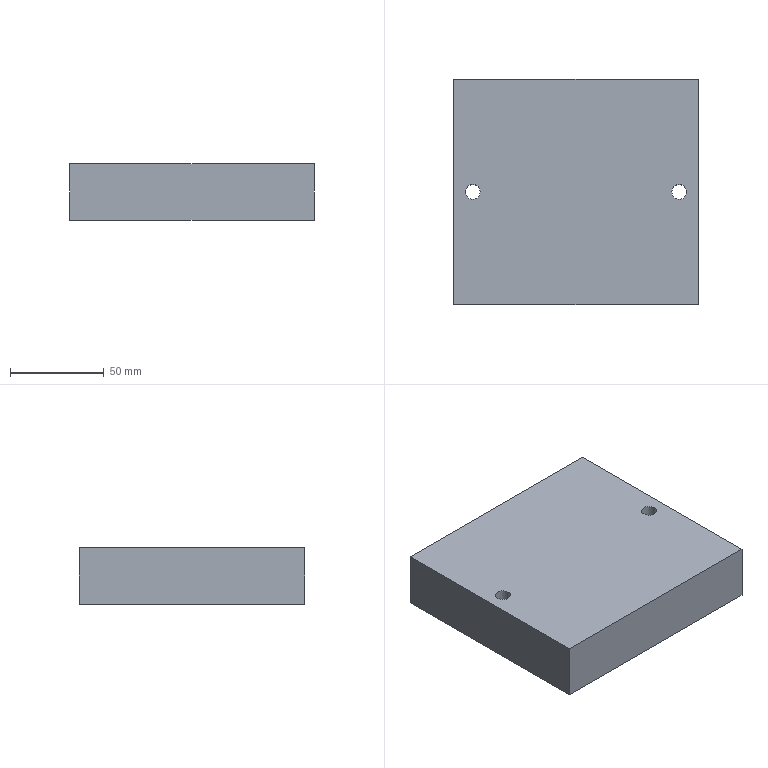Part | STEP file | YBQDJ-YL-7 | 1 solid | 8 faces | box 130 x 120 x 30 mm | volume 464984 mm3 | plane 6 | cylinder 2 | commonest cylinder face diameters 8 x2
STEP:
#1=CARTESIAN_POINT('',(0.,0.,0.));
#2=DIRECTION('',(0.,0.,1.));
#3=DIRECTION('',(1.,0.,0.));
#4=AXIS2_PLACEMENT_3D('',#1,#2,#3);
#5=CARTESIAN_POINT('',(255.5,-195.,95.));
#6=VERTEX_POINT('',#5);
#7=CARTESIAN_POINT('',(247.5,-195.,95.));
#8=VERTEX_POINT('',#7);
#9=CARTESIAN_POINT('',(251.5,-195.,95.));
#10=DIRECTION('',(0.,0.,-1.));
#11=DIRECTION('',(1.,0.,0.));
#12=AXIS2_PLACEMENT_3D('',#9,#10,#11);
#13=CIRCLE('',#12,4.);
#14=CARTESIAN_POINT('',(251.5,-195.,28.));
#15=DIRECTION('',(0.,0.,1.));
#16=DIRECTION('',(-1.,0.,0.));
#17=AXIS2_PLACEMENT_3D('',#14,#15,#16);
#18=CYLINDRICAL_SURFACE('',#17,4.);
#19=CARTESIAN_POINT('',(3.142,67.));
#20=DIRECTION('',(-1.,0.));
#21=VECTOR('',#20,1.);
#22=LINE('',#19,#21);
#23=(GEOMETRIC_REPRESENTATION_CONTEXT(2)PARAMETRIC_REPRESENTATION_CONTEXT()REPRESENTATION_CONTEXT('',''));
#24=DEFINITIONAL_REPRESENTATION('',(#22),#23);
#25=PCURVE('',#18,#24);
#26=CARTESIAN_POINT('',(343.5,-115.,95.));
#27=DIRECTION('',(0.,0.,1.));
#28=DIRECTION('',(1.,0.,0.));
#29=AXIS2_PLACEMENT_3D('',#26,#27,#28);
#30=PLANE('',#29);
#31=CARTESIAN_POINT('',(-88.,-80.));
#32=CARTESIAN_POINT('',(-88.,-86.928));
#33=CARTESIAN_POINT('',(-94.,-83.464));
#34=CARTESIAN_POINT('',(-100.,-80.));
#35=CARTESIAN_POINT('',(-94.,-76.536));
#36=CARTESIAN_POINT('',(-88.,-73.072));
#37=CARTESIAN_POINT('',(-88.,-80.));
#38=(BOUNDED_CURVE()B_SPLINE_CURVE(2,(#31,#32,#33,#34,#35,#36,#37),.UNSPECIFIED.,.T.,.F.)B_SPLINE_CURVE_WITH_KNOTS((1,2,2,2,2,1),(-2.094,0.,2.094,4.189,6.283,8.378),.UNSPECIFIED.)CURVE()GEOMETRIC_REPRESENTATION_ITEM()RATIONAL_B_SPLINE_CURVE((1.,0.5,1.,0.5,1.,0.5,1.))REPRESENTATION_ITEM(''));
#39=(GEOMETRIC_REPRESENTATION_CONTEXT(2)PARAMETRIC_REPRESENTATION_CONTEXT()REPRESENTATION_CONTEXT('',''));
#40=DEFINITIONAL_REPRESENTATION('',(#38),#39);
#41=PCURVE('',#30,#40);
#42=SURFACE_CURVE('',#13,(#25,#41),.PCURVE_S1.);
#43=EDGE_CURVE('',#6,#8,#42,.T.);
#44=ORIENTED_EDGE('',*,*,#43,.T.);
#45=CARTESIAN_POINT('',(247.5,-195.,65.));
#46=VERTEX_POINT('',#45);
#47=CARTESIAN_POINT('',(247.5,-195.,65.));
#48=CARTESIAN_POINT('',(247.5,-195.,95.));
#49=B_SPLINE_CURVE_WITH_KNOTS('',1,(#47,#48),.UNSPECIFIED.,.F.,.F.,(2,2),(37.,67.),.PIECEWISE_BEZIER_KNOTS.);
#50=CARTESIAN_POINT('',(0.,0.));
#51=DIRECTION('',(0.,1.));
#52=VECTOR('',#51,1.);
#53=LINE('',#50,#52);
#54=(GEOMETRIC_REPRESENTATION_CONTEXT(2)PARAMETRIC_REPRESENTATION_CONTEXT()REPRESENTATION_CONTEXT('',''));
#55=DEFINITIONAL_REPRESENTATION('',(#53),#54);
#56=PCURVE('',#18,#55);
#57=CARTESIAN_POINT('',(6.283,0.));
#58=DIRECTION('',(0.,1.));
#59=VECTOR('',#58,1.);
#60=LINE('',#57,#59);
#61=(GEOMETRIC_REPRESENTATION_CONTEXT(2)PARAMETRIC_REPRESENTATION_CONTEXT()REPRESENTATION_CONTEXT('',''));
#62=DEFINITIONAL_REPRESENTATION('',(#60),#61);
#63=PCURVE('',#18,#62);
#64=SEAM_CURVE('',#49,(#56,#63),.PCURVE_S1.);
#65=EDGE_CURVE('',#46,#8,#64,.T.);
#66=ORIENTED_EDGE('',*,*,#65,.F.);
#67=CARTESIAN_POINT('',(251.5,-195.,65.));
#68=DIRECTION('',(0.,0.,1.));
#69=DIRECTION('',(-1.,0.,0.));
#70=AXIS2_PLACEMENT_3D('',#67,#68,#69);
#71=CIRCLE('',#70,4.);
#72=CARTESIAN_POINT('',(0.,37.));
#73=DIRECTION('',(1.,0.));
#74=VECTOR('',#73,1.);
#75=LINE('',#72,#74);
#76=(GEOMETRIC_REPRESENTATION_CONTEXT(2)PARAMETRIC_REPRESENTATION_CONTEXT()REPRESENTATION_CONTEXT('',''));
#77=DEFINITIONAL_REPRESENTATION('',(#75),#76);
#78=PCURVE('',#18,#77);
#79=CARTESIAN_POINT('',(343.5,-115.,65.));
#80=DIRECTION('',(0.,0.,1.));
#81=DIRECTION('',(1.,0.,0.));
#82=AXIS2_PLACEMENT_3D('',#79,#80,#81);
#83=PLANE('',#82);
#84=CARTESIAN_POINT('',(-92.,-80.));
#85=DIRECTION('',(-1.,0.));
#86=AXIS2_PLACEMENT_2D('',#84,#85);
#87=CIRCLE('',#86,4.);
#88=(GEOMETRIC_REPRESENTATION_CONTEXT(2)PARAMETRIC_REPRESENTATION_CONTEXT()REPRESENTATION_CONTEXT('',''));
#89=DEFINITIONAL_REPRESENTATION('',(#87),#88);
#90=PCURVE('',#83,#89);
#91=SURFACE_CURVE('',#71,(#78,#90),.PCURVE_S1.);
#92=EDGE_CURVE('',#46,#46,#91,.T.);
#93=ORIENTED_EDGE('',*,*,#92,.T.);
#94=ORIENTED_EDGE('',*,*,#65,.T.);
#95=CARTESIAN_POINT('',(251.5,-195.,95.));
#96=DIRECTION('',(0.,0.,-1.));
#97=DIRECTION('',(1.,0.,0.));
#98=AXIS2_PLACEMENT_3D('',#95,#96,#97);
#99=CIRCLE('',#98,4.);
#100=CARTESIAN_POINT('',(9.425,67.));
#101=DIRECTION('',(-1.,0.));
#102=VECTOR('',#101,1.);
#103=LINE('',#100,#102);
#104=(GEOMETRIC_REPRESENTATION_CONTEXT(2)PARAMETRIC_REPRESENTATION_CONTEXT()REPRESENTATION_CONTEXT('',''));
#105=DEFINITIONAL_REPRESENTATION('',(#103),#104);
#106=PCURVE('',#18,#105);
#107=CARTESIAN_POINT('',(-88.,-80.));
#108=CARTESIAN_POINT('',(-88.,-86.928));
#109=CARTESIAN_POINT('',(-94.,-83.464));
#110=CARTESIAN_POINT('',(-100.,-80.));
#111=CARTESIAN_POINT('',(-94.,-76.536));
#112=CARTESIAN_POINT('',(-88.,-73.072));
#113=CARTESIAN_POINT('',(-88.,-80.));
#114=(BOUNDED_CURVE()B_SPLINE_CURVE(2,(#107,#108,#109,#110,#111,#112,#113),.UNSPECIFIED.,.T.,.F.)B_SPLINE_CURVE_WITH_KNOTS((1,2,2,2,2,1),(-2.094,0.,2.094,4.189,6.283,8.378),.UNSPECIFIED.)CURVE()GEOMETRIC_REPRESENTATION_ITEM()RATIONAL_B_SPLINE_CURVE((1.,0.5,1.,0.5,1.,0.5,1.))REPRESENTATION_ITEM(''));
#115=(GEOMETRIC_REPRESENTATION_CONTEXT(2)PARAMETRIC_REPRESENTATION_CONTEXT()REPRESENTATION_CONTEXT('',''));
#116=DEFINITIONAL_REPRESENTATION('',(#114),#115);
#117=PCURVE('',#30,#116);
#118=SURFACE_CURVE('',#99,(#106,#117),.PCURVE_S1.);
#119=EDGE_CURVE('',#8,#6,#118,.T.);
#120=ORIENTED_EDGE('',*,*,#119,.T.);
#121=EDGE_LOOP('',(#44,#66,#93,#94,#120));
#122=FACE_BOUND('',#121,.F.);
#123=ADVANCED_FACE('',(#122),#18,.F.);
#124=CARTESIAN_POINT('',(241.5,-135.,95.));
#125=VERTEX_POINT('',#124);
#126=CARTESIAN_POINT('',(241.5,-135.,65.));
#127=VERTEX_POINT('',#126);
#128=CARTESIAN_POINT('',(241.5,-135.,108.));
#129=DIRECTION('',(0.,0.,-1.));
#130=VECTOR('',#129,1.);
#131=LINE('',#128,#130);
#132=CARTESIAN_POINT('',(241.5,-90.,108.));
#133=DIRECTION('',(1.,0.,0.));
#134=DIRECTION('',(0.,0.,-1.));
#135=AXIS2_PLACEMENT_3D('',#132,#133,#134);
#136=PLANE('',#135);
#137=CARTESIAN_POINT('',(0.,-45.));
#138=DIRECTION('',(1.,0.));
#139=VECTOR('',#138,1.);
#140=LINE('',#137,#139);
#141=(GEOMETRIC_REPRESENTATION_CONTEXT(2)PARAMETRIC_REPRESENTATION_CONTEXT()REPRESENTATION_CONTEXT('',''));
#142=DEFINITIONAL_REPRESENTATION('',(#140),#141);
#143=PCURVE('',#136,#142);
#144=CARTESIAN_POINT('',(343.5,-135.,88.));
#145=DIRECTION('',(0.,1.,0.));
#146=DIRECTION('',(-1.,0.,0.));
#147=AXIS2_PLACEMENT_3D('',#144,#145,#146);
#148=PLANE('',#147);
#149=CARTESIAN_POINT('',(102.,20.));
#150=DIRECTION('',(0.,-1.));
#151=VECTOR('',#150,1.);
#152=LINE('',#149,#151);
#153=(GEOMETRIC_REPRESENTATION_CONTEXT(2)PARAMETRIC_REPRESENTATION_CONTEXT()REPRESENTATION_CONTEXT('',''));
#154=DEFINITIONAL_REPRESENTATION('',(#152),#153);
#155=PCURVE('',#148,#154);
#156=SURFACE_CURVE('',#131,(#143,#155),.PCURVE_S1.);
#157=EDGE_CURVE('',#125,#127,#156,.T.);
#158=ORIENTED_EDGE('',*,*,#157,.T.);
#159=CARTESIAN_POINT('',(241.5,-255.,65.));
#160=VERTEX_POINT('',#159);
#161=CARTESIAN_POINT('',(241.5,-90.,65.));
#162=DIRECTION('',(0.,-1.,0.));
#163=VECTOR('',#162,1.);
#164=LINE('',#161,#163);
#165=CARTESIAN_POINT('',(43.,0.));
#166=DIRECTION('',(0.,-1.));
#167=VECTOR('',#166,1.);
#168=LINE('',#165,#167);
#169=(GEOMETRIC_REPRESENTATION_CONTEXT(2)PARAMETRIC_REPRESENTATION_CONTEXT()REPRESENTATION_CONTEXT('',''));
#170=DEFINITIONAL_REPRESENTATION('',(#168),#169);
#171=PCURVE('',#136,#170);
#172=CARTESIAN_POINT('',(-102.,25.));
#173=DIRECTION('',(0.,-1.));
#174=VECTOR('',#173,1.);
#175=LINE('',#172,#174);
#176=(GEOMETRIC_REPRESENTATION_CONTEXT(2)PARAMETRIC_REPRESENTATION_CONTEXT()REPRESENTATION_CONTEXT('',''));
#177=DEFINITIONAL_REPRESENTATION('',(#175),#176);
#178=PCURVE('',#83,#177);
#179=SURFACE_CURVE('',#164,(#171,#178),.PCURVE_S1.);
#180=EDGE_CURVE('',#127,#160,#179,.T.);
#181=ORIENTED_EDGE('',*,*,#180,.T.);
#182=CARTESIAN_POINT('',(241.5,-255.,95.));
#183=VERTEX_POINT('',#182);
#184=CARTESIAN_POINT('',(241.5,-255.,88.));
#185=DIRECTION('',(0.,0.,-1.));
#186=VECTOR('',#185,1.);
#187=LINE('',#184,#186);
#188=CARTESIAN_POINT('',(20.,-165.));
#189=DIRECTION('',(1.,0.));
#190=VECTOR('',#189,1.);
#191=LINE('',#188,#190);
#192=(GEOMETRIC_REPRESENTATION_CONTEXT(2)PARAMETRIC_REPRESENTATION_CONTEXT()REPRESENTATION_CONTEXT('',''));
#193=DEFINITIONAL_REPRESENTATION('',(#191),#192);
#194=PCURVE('',#136,#193);
#195=CARTESIAN_POINT('',(343.5,-255.,88.));
#196=DIRECTION('',(0.,1.,0.));
#197=DIRECTION('',(-1.,0.,0.));
#198=AXIS2_PLACEMENT_3D('',#195,#196,#197);
#199=PLANE('',#198);
#200=CARTESIAN_POINT('',(102.,0.));
#201=DIRECTION('',(0.,-1.));
#202=VECTOR('',#201,1.);
#203=LINE('',#200,#202);
#204=(GEOMETRIC_REPRESENTATION_CONTEXT(2)PARAMETRIC_REPRESENTATION_CONTEXT()REPRESENTATION_CONTEXT('',''));
#205=DEFINITIONAL_REPRESENTATION('',(#203),#204);
#206=PCURVE('',#199,#205);
#207=SURFACE_CURVE('',#187,(#194,#206),.PCURVE_S1.);
#208=EDGE_CURVE('',#183,#160,#207,.T.);
#209=ORIENTED_EDGE('',*,*,#208,.F.);
#210=CARTESIAN_POINT('',(241.5,-90.,95.));
#211=DIRECTION('',(0.,-1.,0.));
#212=VECTOR('',#211,1.);
#213=LINE('',#210,#212);
#214=CARTESIAN_POINT('',(13.,0.));
#215=DIRECTION('',(0.,-1.));
#216=VECTOR('',#215,1.);
#217=LINE('',#214,#216);
#218=(GEOMETRIC_REPRESENTATION_CONTEXT(2)PARAMETRIC_REPRESENTATION_CONTEXT()REPRESENTATION_CONTEXT('',''));
#219=DEFINITIONAL_REPRESENTATION('',(#217),#218);
#220=PCURVE('',#136,#219);
#221=CARTESIAN_POINT('',(-102.,25.));
#222=DIRECTION('',(0.,-1.));
#223=VECTOR('',#222,1.);
#224=LINE('',#221,#223);
#225=(GEOMETRIC_REPRESENTATION_CONTEXT(2)PARAMETRIC_REPRESENTATION_CONTEXT()REPRESENTATION_CONTEXT('',''));
#226=DEFINITIONAL_REPRESENTATION('',(#224),#225);
#227=PCURVE('',#30,#226);
#228=SURFACE_CURVE('',#213,(#220,#227),.PCURVE_S1.);
#229=EDGE_CURVE('',#125,#183,#228,.T.);
#230=ORIENTED_EDGE('',*,*,#229,.F.);
#231=EDGE_LOOP('',(#158,#181,#209,#230));
#232=FACE_BOUND('',#231,.T.);
#233=ADVANCED_FACE('',(#232),#136,.F.);
#234=CARTESIAN_POINT('',(371.5,-135.,95.));
#235=VERTEX_POINT('',#234);
#236=CARTESIAN_POINT('',(371.5,-135.,65.));
#237=VERTEX_POINT('',#236);
#238=CARTESIAN_POINT('',(371.5,-135.,88.));
#239=DIRECTION('',(0.,0.,-1.));
#240=VECTOR('',#239,1.);
#241=LINE('',#238,#240);
#242=CARTESIAN_POINT('',(-28.,0.));
#243=DIRECTION('',(0.,-1.));
#244=VECTOR('',#243,1.);
#245=LINE('',#242,#244);
#246=(GEOMETRIC_REPRESENTATION_CONTEXT(2)PARAMETRIC_REPRESENTATION_CONTEXT()REPRESENTATION_CONTEXT('',''));
#247=DEFINITIONAL_REPRESENTATION('',(#245),#246);
#248=PCURVE('',#148,#247);
#249=CARTESIAN_POINT('',(371.5,-300.,108.));
#250=DIRECTION('',(-1.,0.,0.));
#251=DIRECTION('',(0.,0.,1.));
#252=AXIS2_PLACEMENT_3D('',#249,#250,#251);
#253=PLANE('',#252);
#254=CARTESIAN_POINT('',(-20.,165.));
#255=DIRECTION('',(-1.,0.));
#256=VECTOR('',#255,1.);
#257=LINE('',#254,#256);
#258=(GEOMETRIC_REPRESENTATION_CONTEXT(2)PARAMETRIC_REPRESENTATION_CONTEXT()REPRESENTATION_CONTEXT('',''));
#259=DEFINITIONAL_REPRESENTATION('',(#257),#258);
#260=PCURVE('',#253,#259);
#261=SURFACE_CURVE('',#241,(#248,#260),.PCURVE_S1.);
#262=EDGE_CURVE('',#235,#237,#261,.T.);
#263=ORIENTED_EDGE('',*,*,#262,.T.);
#264=CARTESIAN_POINT('',(343.5,-135.,65.));
#265=DIRECTION('',(-1.,0.,0.));
#266=VECTOR('',#265,1.);
#267=LINE('',#264,#266);
#268=CARTESIAN_POINT('',(0.,-23.));
#269=DIRECTION('',(1.,0.));
#270=VECTOR('',#269,1.);
#271=LINE('',#268,#270);
#272=(GEOMETRIC_REPRESENTATION_CONTEXT(2)PARAMETRIC_REPRESENTATION_CONTEXT()REPRESENTATION_CONTEXT('',''));
#273=DEFINITIONAL_REPRESENTATION('',(#271),#272);
#274=PCURVE('',#148,#273);
#275=CARTESIAN_POINT('',(0.,-20.));
#276=DIRECTION('',(-1.,0.));
#277=VECTOR('',#276,1.);
#278=LINE('',#275,#277);
#279=(GEOMETRIC_REPRESENTATION_CONTEXT(2)PARAMETRIC_REPRESENTATION_CONTEXT()REPRESENTATION_CONTEXT('',''));
#280=DEFINITIONAL_REPRESENTATION('',(#278),#279);
#281=PCURVE('',#83,#280);
#282=SURFACE_CURVE('',#267,(#274,#281),.PCURVE_S1.);
#283=EDGE_CURVE('',#237,#127,#282,.T.);
#284=ORIENTED_EDGE('',*,*,#283,.T.);
#285=ORIENTED_EDGE('',*,*,#157,.F.);
#286=CARTESIAN_POINT('',(343.5,-135.,95.));
#287=DIRECTION('',(-1.,0.,0.));
#288=VECTOR('',#287,1.);
#289=LINE('',#286,#288);
#290=CARTESIAN_POINT('',(0.,7.));
#291=DIRECTION('',(1.,0.));
#292=VECTOR('',#291,1.);
#293=LINE('',#290,#292);
#294=(GEOMETRIC_REPRESENTATION_CONTEXT(2)PARAMETRIC_REPRESENTATION_CONTEXT()REPRESENTATION_CONTEXT('',''));
#295=DEFINITIONAL_REPRESENTATION('',(#293),#294);
#296=PCURVE('',#148,#295);
#297=CARTESIAN_POINT('',(0.,-20.));
#298=DIRECTION('',(-1.,0.));
#299=VECTOR('',#298,1.);
#300=LINE('',#297,#299);
#301=(GEOMETRIC_REPRESENTATION_CONTEXT(2)PARAMETRIC_REPRESENTATION_CONTEXT()REPRESENTATION_CONTEXT('',''));
#302=DEFINITIONAL_REPRESENTATION('',(#300),#301);
#303=PCURVE('',#30,#302);
#304=SURFACE_CURVE('',#289,(#296,#303),.PCURVE_S1.);
#305=EDGE_CURVE('',#235,#125,#304,.T.);
#306=ORIENTED_EDGE('',*,*,#305,.F.);
#307=EDGE_LOOP('',(#263,#284,#285,#306));
#308=FACE_BOUND('',#307,.T.);
#309=ADVANCED_FACE('',(#308),#148,.T.);
#310=CARTESIAN_POINT('',(371.5,-255.,95.));
#311=VERTEX_POINT('',#310);
#312=CARTESIAN_POINT('',(371.5,-115.,95.));
#313=DIRECTION('',(0.,-1.,0.));
#314=VECTOR('',#313,1.);
#315=LINE('',#312,#314);
#316=CARTESIAN_POINT('',(-13.,185.));
#317=DIRECTION('',(0.,-1.));
#318=VECTOR('',#317,1.);
#319=LINE('',#316,#318);
#320=(GEOMETRIC_REPRESENTATION_CONTEXT(2)PARAMETRIC_REPRESENTATION_CONTEXT()REPRESENTATION_CONTEXT('',''));
#321=DEFINITIONAL_REPRESENTATION('',(#319),#320);
#322=PCURVE('',#253,#321);
#323=CARTESIAN_POINT('',(28.,0.));
#324=DIRECTION('',(0.,-1.));
#325=VECTOR('',#324,1.);
#326=LINE('',#323,#325);
#327=(GEOMETRIC_REPRESENTATION_CONTEXT(2)PARAMETRIC_REPRESENTATION_CONTEXT()REPRESENTATION_CONTEXT('',''));
#328=DEFINITIONAL_REPRESENTATION('',(#326),#327);
#329=PCURVE('',#30,#328);
#330=SURFACE_CURVE('',#315,(#322,#329),.PCURVE_S1.);
#331=EDGE_CURVE('',#235,#311,#330,.T.);
#332=ORIENTED_EDGE('',*,*,#331,.T.);
#333=CARTESIAN_POINT('',(371.5,-255.,65.));
#334=VERTEX_POINT('',#333);
#335=CARTESIAN_POINT('',(371.5,-255.,108.));
#336=DIRECTION('',(0.,0.,-1.));
#337=VECTOR('',#336,1.);
#338=LINE('',#335,#337);
#339=CARTESIAN_POINT('',(0.,45.));
#340=DIRECTION('',(-1.,0.));
#341=VECTOR('',#340,1.);
#342=LINE('',#339,#341);
#343=(GEOMETRIC_REPRESENTATION_CONTEXT(2)PARAMETRIC_REPRESENTATION_CONTEXT()REPRESENTATION_CONTEXT('',''));
#344=DEFINITIONAL_REPRESENTATION('',(#342),#343);
#345=PCURVE('',#253,#344);
#346=CARTESIAN_POINT('',(-28.,20.));
#347=DIRECTION('',(0.,-1.));
#348=VECTOR('',#347,1.);
#349=LINE('',#346,#348);
#350=(GEOMETRIC_REPRESENTATION_CONTEXT(2)PARAMETRIC_REPRESENTATION_CONTEXT()REPRESENTATION_CONTEXT('',''));
#351=DEFINITIONAL_REPRESENTATION('',(#349),#350);
#352=PCURVE('',#199,#351);
#353=SURFACE_CURVE('',#338,(#345,#352),.PCURVE_S1.);
#354=EDGE_CURVE('',#311,#334,#353,.T.);
#355=ORIENTED_EDGE('',*,*,#354,.T.);
#356=CARTESIAN_POINT('',(371.5,-115.,65.));
#357=DIRECTION('',(0.,-1.,0.));
#358=VECTOR('',#357,1.);
#359=LINE('',#356,#358);
#360=CARTESIAN_POINT('',(-43.,185.));
#361=DIRECTION('',(0.,-1.));
#362=VECTOR('',#361,1.);
#363=LINE('',#360,#362);
#364=(GEOMETRIC_REPRESENTATION_CONTEXT(2)PARAMETRIC_REPRESENTATION_CONTEXT()REPRESENTATION_CONTEXT('',''));
#365=DEFINITIONAL_REPRESENTATION('',(#363),#364);
#366=PCURVE('',#253,#365);
#367=CARTESIAN_POINT('',(28.,0.));
#368=DIRECTION('',(0.,-1.));
#369=VECTOR('',#368,1.);
#370=LINE('',#367,#369);
#371=(GEOMETRIC_REPRESENTATION_CONTEXT(2)PARAMETRIC_REPRESENTATION_CONTEXT()REPRESENTATION_CONTEXT('',''));
#372=DEFINITIONAL_REPRESENTATION('',(#370),#371);
#373=PCURVE('',#83,#372);
#374=SURFACE_CURVE('',#359,(#366,#373),.PCURVE_S1.);
#375=EDGE_CURVE('',#237,#334,#374,.T.);
#376=ORIENTED_EDGE('',*,*,#375,.F.);
#377=ORIENTED_EDGE('',*,*,#262,.F.);
#378=EDGE_LOOP('',(#332,#355,#376,#377));
#379=FACE_BOUND('',#378,.T.);
#380=ADVANCED_FACE('',(#379),#253,.F.);
#381=ORIENTED_EDGE('',*,*,#208,.T.);
#382=CARTESIAN_POINT('',(343.5,-255.,65.));
#383=DIRECTION('',(-1.,0.,0.));
#384=VECTOR('',#383,1.);
#385=LINE('',#382,#384);
#386=CARTESIAN_POINT('',(0.,-23.));
#387=DIRECTION('',(1.,0.));
#388=VECTOR('',#387,1.);
#389=LINE('',#386,#388);
#390=(GEOMETRIC_REPRESENTATION_CONTEXT(2)PARAMETRIC_REPRESENTATION_CONTEXT()REPRESENTATION_CONTEXT('',''));
#391=DEFINITIONAL_REPRESENTATION('',(#389),#390);
#392=PCURVE('',#199,#391);
#393=CARTESIAN_POINT('',(0.,-140.));
#394=DIRECTION('',(-1.,0.));
#395=VECTOR('',#394,1.);
#396=LINE('',#393,#395);
#397=(GEOMETRIC_REPRESENTATION_CONTEXT(2)PARAMETRIC_REPRESENTATION_CONTEXT()REPRESENTATION_CONTEXT('',''));
#398=DEFINITIONAL_REPRESENTATION('',(#396),#397);
#399=PCURVE('',#83,#398);
#400=SURFACE_CURVE('',#385,(#392,#399),.PCURVE_S1.);
#401=EDGE_CURVE('',#334,#160,#400,.T.);
#402=ORIENTED_EDGE('',*,*,#401,.F.);
#403=ORIENTED_EDGE('',*,*,#354,.F.);
#404=CARTESIAN_POINT('',(343.5,-255.,95.));
#405=DIRECTION('',(-1.,0.,0.));
#406=VECTOR('',#405,1.);
#407=LINE('',#404,#406);
#408=CARTESIAN_POINT('',(0.,7.));
#409=DIRECTION('',(1.,0.));
#410=VECTOR('',#409,1.);
#411=LINE('',#408,#410);
#412=(GEOMETRIC_REPRESENTATION_CONTEXT(2)PARAMETRIC_REPRESENTATION_CONTEXT()REPRESENTATION_CONTEXT('',''));
#413=DEFINITIONAL_REPRESENTATION('',(#411),#412);
#414=PCURVE('',#199,#413);
#415=CARTESIAN_POINT('',(0.,-140.));
#416=DIRECTION('',(-1.,0.));
#417=VECTOR('',#416,1.);
#418=LINE('',#415,#417);
#419=(GEOMETRIC_REPRESENTATION_CONTEXT(2)PARAMETRIC_REPRESENTATION_CONTEXT()REPRESENTATION_CONTEXT('',''));
#420=DEFINITIONAL_REPRESENTATION('',(#418),#419);
#421=PCURVE('',#30,#420);
#422=SURFACE_CURVE('',#407,(#414,#421),.PCURVE_S1.);
#423=EDGE_CURVE('',#311,#183,#422,.T.);
#424=ORIENTED_EDGE('',*,*,#423,.T.);
#425=EDGE_LOOP('',(#381,#402,#403,#424));
#426=FACE_BOUND('',#425,.T.);
#427=ADVANCED_FACE('',(#426),#199,.F.);
#428=CARTESIAN_POINT('',(365.5,-195.,95.));
#429=VERTEX_POINT('',#428);
#430=CARTESIAN_POINT('',(361.5,-195.,95.));
#431=DIRECTION('',(0.,0.,1.));
#432=DIRECTION('',(1.,0.,0.));
#433=AXIS2_PLACEMENT_3D('',#430,#431,#432);
#434=CIRCLE('',#433,4.);
#435=CARTESIAN_POINT('',(361.5,-195.,28.));
#436=DIRECTION('',(0.,0.,1.));
#437=DIRECTION('',(1.,0.,0.));
#438=AXIS2_PLACEMENT_3D('',#435,#436,#437);
#439=CYLINDRICAL_SURFACE('',#438,4.);
#440=CARTESIAN_POINT('',(0.,67.));
#441=DIRECTION('',(1.,0.));
#442=VECTOR('',#441,1.);
#443=LINE('',#440,#442);
#444=(GEOMETRIC_REPRESENTATION_CONTEXT(2)PARAMETRIC_REPRESENTATION_CONTEXT()REPRESENTATION_CONTEXT('',''));
#445=DEFINITIONAL_REPRESENTATION('',(#443),#444);
#446=PCURVE('',#439,#445);
#447=CARTESIAN_POINT('',(18.,-80.));
#448=DIRECTION('',(1.,0.));
#449=AXIS2_PLACEMENT_2D('',#447,#448);
#450=CIRCLE('',#449,4.);
#451=(GEOMETRIC_REPRESENTATION_CONTEXT(2)PARAMETRIC_REPRESENTATION_CONTEXT()REPRESENTATION_CONTEXT('',''));
#452=DEFINITIONAL_REPRESENTATION('',(#450),#451);
#453=PCURVE('',#30,#452);
#454=SURFACE_CURVE('',#434,(#446,#453),.PCURVE_S1.);
#455=EDGE_CURVE('',#429,#429,#454,.T.);
#456=ORIENTED_EDGE('',*,*,#455,.F.);
#457=CARTESIAN_POINT('',(365.5,-195.,65.));
#458=VERTEX_POINT('',#457);
#459=CARTESIAN_POINT('',(365.5,-195.,65.));
#460=CARTESIAN_POINT('',(365.5,-195.,95.));
#461=B_SPLINE_CURVE_WITH_KNOTS('',1,(#459,#460),.UNSPECIFIED.,.F.,.F.,(2,2),(37.,67.),.PIECEWISE_BEZIER_KNOTS.);
#462=CARTESIAN_POINT('',(0.,0.));
#463=DIRECTION('',(0.,1.));
#464=VECTOR('',#463,1.);
#465=LINE('',#462,#464);
#466=(GEOMETRIC_REPRESENTATION_CONTEXT(2)PARAMETRIC_REPRESENTATION_CONTEXT()REPRESENTATION_CONTEXT('',''));
#467=DEFINITIONAL_REPRESENTATION('',(#465),#466);
#468=PCURVE('',#439,#467);
#469=CARTESIAN_POINT('',(6.283,0.));
#470=DIRECTION('',(0.,1.));
#471=VECTOR('',#470,1.);
#472=LINE('',#469,#471);
#473=(GEOMETRIC_REPRESENTATION_CONTEXT(2)PARAMETRIC_REPRESENTATION_CONTEXT()REPRESENTATION_CONTEXT('',''));
#474=DEFINITIONAL_REPRESENTATION('',(#472),#473);
#475=PCURVE('',#439,#474);
#476=SEAM_CURVE('',#461,(#468,#475),.PCURVE_S1.);
#477=EDGE_CURVE('',#458,#429,#476,.T.);
#478=ORIENTED_EDGE('',*,*,#477,.F.);
#479=CARTESIAN_POINT('',(361.5,-195.,65.));
#480=DIRECTION('',(0.,0.,1.));
#481=DIRECTION('',(1.,0.,0.));
#482=AXIS2_PLACEMENT_3D('',#479,#480,#481);
#483=CIRCLE('',#482,4.);
#484=CARTESIAN_POINT('',(0.,37.));
#485=DIRECTION('',(1.,0.));
#486=VECTOR('',#485,1.);
#487=LINE('',#484,#486);
#488=(GEOMETRIC_REPRESENTATION_CONTEXT(2)PARAMETRIC_REPRESENTATION_CONTEXT()REPRESENTATION_CONTEXT('',''));
#489=DEFINITIONAL_REPRESENTATION('',(#487),#488);
#490=PCURVE('',#439,#489);
#491=CARTESIAN_POINT('',(18.,-80.));
#492=DIRECTION('',(1.,0.));
#493=AXIS2_PLACEMENT_2D('',#491,#492);
#494=CIRCLE('',#493,4.);
#495=(GEOMETRIC_REPRESENTATION_CONTEXT(2)PARAMETRIC_REPRESENTATION_CONTEXT()REPRESENTATION_CONTEXT('',''));
#496=DEFINITIONAL_REPRESENTATION('',(#494),#495);
#497=PCURVE('',#83,#496);
#498=SURFACE_CURVE('',#483,(#490,#497),.PCURVE_S1.);
#499=EDGE_CURVE('',#458,#458,#498,.T.);
#500=ORIENTED_EDGE('',*,*,#499,.T.);
#501=ORIENTED_EDGE('',*,*,#477,.T.);
#502=EDGE_LOOP('',(#456,#478,#500,#501));
#503=FACE_BOUND('',#502,.F.);
#504=ADVANCED_FACE('',(#503),#439,.F.);
#505=ORIENTED_EDGE('',*,*,#43,.T.);
#506=ORIENTED_EDGE('',*,*,#119,.T.);
#507=EDGE_LOOP('',(#505,#506));
#508=FACE_BOUND('',#507,.T.);
#509=ORIENTED_EDGE('',*,*,#455,.F.);
#510=EDGE_LOOP('',(#509));
#511=FACE_BOUND('',#510,.T.);
#512=ORIENTED_EDGE('',*,*,#423,.F.);
#513=ORIENTED_EDGE('',*,*,#331,.F.);
#514=ORIENTED_EDGE('',*,*,#305,.T.);
#515=ORIENTED_EDGE('',*,*,#229,.T.);
#516=EDGE_LOOP('',(#512,#513,#514,#515));
#517=FACE_BOUND('',#516,.T.);
#518=ADVANCED_FACE('',(#508,#511,#517),#30,.T.);
#519=ORIENTED_EDGE('',*,*,#92,.T.);
#520=EDGE_LOOP('',(#519));
#521=FACE_BOUND('',#520,.T.);
#522=ORIENTED_EDGE('',*,*,#499,.T.);
#523=EDGE_LOOP('',(#522));
#524=FACE_BOUND('',#523,.T.);
#525=ORIENTED_EDGE('',*,*,#401,.T.);
#526=ORIENTED_EDGE('',*,*,#180,.F.);
#527=ORIENTED_EDGE('',*,*,#283,.F.);
#528=ORIENTED_EDGE('',*,*,#375,.T.);
#529=EDGE_LOOP('',(#525,#526,#527,#528));
#530=FACE_BOUND('',#529,.T.);
#531=ADVANCED_FACE('',(#521,#524,#530),#83,.F.);
#532=CLOSED_SHELL('',(#123,#233,#309,#380,#427,#504,#518,#531));
#533=MANIFOLD_SOLID_BREP('',#532);
#534=(LENGTH_UNIT()NAMED_UNIT(*)SI_UNIT(.MILLI.,.METRE.));
#535=UNCERTAINTY_MEASURE_WITH_UNIT(LENGTH_MEASURE(0.000002),#534,'','');
#536=(NAMED_UNIT(*)PLANE_ANGLE_UNIT()SI_UNIT($,.RADIAN.));
#537=(NAMED_UNIT(*)SI_UNIT($,.STERADIAN.)SOLID_ANGLE_UNIT());
#538=(GEOMETRIC_REPRESENTATION_CONTEXT(3)GLOBAL_UNCERTAINTY_ASSIGNED_CONTEXT((#535))GLOBAL_UNIT_ASSIGNED_CONTEXT((#534,#536,#537))REPRESENTATION_CONTEXT('',''));
#539=ADVANCED_BREP_SHAPE_REPRESENTATION('',(#4,#533),#538);